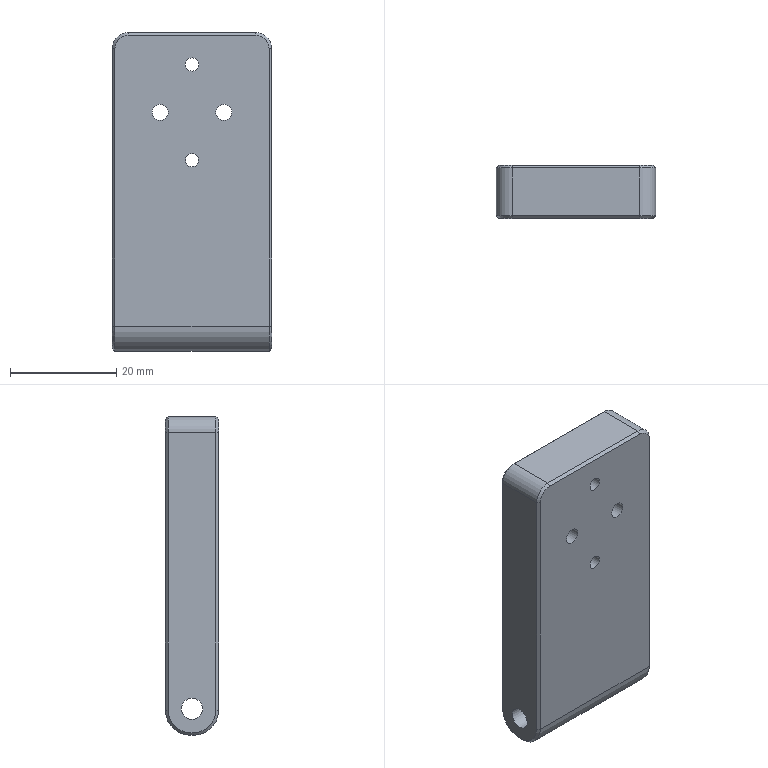Part | NX | 1 solid | 31 faces | box 30 x 10 x 60 mm | volume 17016 mm3 | plane 14 | cylinder 9 | cone 8 | commonest cylinder face diameters 2.5 x2 3 x2 6 x2 9.5 x2 4 x1
STEP:
#1=CARTESIAN_POINT('',(-12.,0.5,30.));
#2=VERTEX_POINT('',#1);
#3=CARTESIAN_POINT('',(-12.,0.,29.5));
#4=VERTEX_POINT('',#3);
#5=CARTESIAN_POINT('',(-12.,0.5,30.));
#6=DIRECTION('',(0.,-0.7071,-0.7071));
#7=VECTOR('',#6,1000.);
#8=LINE('',#5,#7);
#9=EDGE_CURVE('',#2,#4,#8,.T.);
#10=ORIENTED_EDGE('',*,*,#9,.T.);
#11=CARTESIAN_POINT('',(12.,0.,29.5));
#12=VERTEX_POINT('',#11);
#13=CARTESIAN_POINT('',(-12.,0.,29.5));
#14=DIRECTION('',(-1.,0.,0.));
#15=VECTOR('',#14,1000.);
#16=LINE('',#13,#15);
#17=EDGE_CURVE('',#12,#4,#16,.T.);
#18=ORIENTED_EDGE('',*,*,#17,.F.);
#19=CARTESIAN_POINT('',(12.,0.5,30.));
#20=VERTEX_POINT('',#19);
#21=CARTESIAN_POINT('',(12.,0.,29.5));
#22=DIRECTION('',(0.,0.7071,0.7071));
#23=VECTOR('',#22,1000.);
#24=LINE('',#21,#23);
#25=EDGE_CURVE('',#12,#20,#24,.T.);
#26=ORIENTED_EDGE('',*,*,#25,.T.);
#27=CARTESIAN_POINT('',(12.,0.5,30.));
#28=DIRECTION('',(1.,0.,0.));
#29=VECTOR('',#28,1000.);
#30=LINE('',#27,#29);
#31=EDGE_CURVE('',#2,#20,#30,.T.);
#32=ORIENTED_EDGE('',*,*,#31,.F.);
#33=EDGE_LOOP('',(#10,#18,#26,#32));
#34=FACE_BOUND('',#33,.T.);
#35=CARTESIAN_POINT('',(-15.,0.5,30.));
#36=DIRECTION('',(0.,-0.7071,0.7071));
#37=DIRECTION('',(-1.,0.,0.));
#38=AXIS2_PLACEMENT_3D('',#35,#36,#37);
#39=PLANE('',#38);
#40=ADVANCED_FACE('',(#34),#39,.T.);
#41=CARTESIAN_POINT('',(14.5,0.,27.));
#42=VERTEX_POINT('',#41);
#43=CARTESIAN_POINT('',(15.,0.5,27.));
#44=VERTEX_POINT('',#43);
#45=CARTESIAN_POINT('',(14.5,0.,27.));
#46=DIRECTION('',(0.7071,0.7071,0.));
#47=VECTOR('',#46,1000.);
#48=LINE('',#45,#47);
#49=EDGE_CURVE('',#42,#44,#48,.T.);
#50=ORIENTED_EDGE('',*,*,#49,.T.);
#51=CARTESIAN_POINT('',(12.,0.5,27.));
#52=DIRECTION('',(0.,1.,0.));
#53=DIRECTION('',(0.,0.,-1.));
#54=AXIS2_PLACEMENT_3D('',#51,#52,#53);
#55=CIRCLE('',#54,3.);
#56=EDGE_CURVE('',#20,#44,#55,.T.);
#57=ORIENTED_EDGE('',*,*,#56,.F.);
#58=ORIENTED_EDGE('',*,*,#25,.F.);
#59=CARTESIAN_POINT('',(12.,0.,27.));
#60=DIRECTION('',(0.,-1.,0.));
#61=DIRECTION('',(0.,0.,-1.));
#62=AXIS2_PLACEMENT_3D('',#59,#60,#61);
#63=CIRCLE('',#62,2.5);
#64=EDGE_CURVE('',#42,#12,#63,.T.);
#65=ORIENTED_EDGE('',*,*,#64,.F.);
#66=EDGE_LOOP('',(#50,#57,#58,#65));
#67=FACE_BOUND('',#66,.T.);
#68=CARTESIAN_POINT('',(12.,0.,27.));
#69=DIRECTION('',(0.,1.,0.));
#70=DIRECTION('',(0.,0.,1.));
#71=AXIS2_PLACEMENT_3D('',#68,#69,#70);
#72=CONICAL_SURFACE('',#71,2.5,0.7854);
#73=ADVANCED_FACE('',(#67),#72,.T.);
#74=CARTESIAN_POINT('',(-15.,0.5,27.));
#75=VERTEX_POINT('',#74);
#76=CARTESIAN_POINT('',(-14.5,0.,27.));
#77=VERTEX_POINT('',#76);
#78=CARTESIAN_POINT('',(-15.,0.5,27.));
#79=DIRECTION('',(0.7071,-0.7071,0.));
#80=VECTOR('',#79,1000.);
#81=LINE('',#78,#80);
#82=EDGE_CURVE('',#75,#77,#81,.T.);
#83=ORIENTED_EDGE('',*,*,#82,.T.);
#84=CARTESIAN_POINT('',(-12.,0.,27.));
#85=DIRECTION('',(0.,-1.,0.));
#86=DIRECTION('',(0.,0.,-1.));
#87=AXIS2_PLACEMENT_3D('',#84,#85,#86);
#88=CIRCLE('',#87,2.5);
#89=EDGE_CURVE('',#4,#77,#88,.T.);
#90=ORIENTED_EDGE('',*,*,#89,.F.);
#91=ORIENTED_EDGE('',*,*,#9,.F.);
#92=CARTESIAN_POINT('',(-12.,0.5,27.));
#93=DIRECTION('',(0.,1.,0.));
#94=DIRECTION('',(0.,0.,-1.));
#95=AXIS2_PLACEMENT_3D('',#92,#93,#94);
#96=CIRCLE('',#95,3.);
#97=EDGE_CURVE('',#75,#2,#96,.T.);
#98=ORIENTED_EDGE('',*,*,#97,.F.);
#99=EDGE_LOOP('',(#83,#90,#91,#98));
#100=FACE_BOUND('',#99,.T.);
#101=CARTESIAN_POINT('',(-12.,0.,27.));
#102=DIRECTION('',(0.,1.,0.));
#103=DIRECTION('',(0.,0.,1.));
#104=AXIS2_PLACEMENT_3D('',#101,#102,#103);
#105=CONICAL_SURFACE('',#104,2.5,0.7854);
#106=ADVANCED_FACE('',(#100),#105,.T.);
#107=CARTESIAN_POINT('',(14.5,0.,-25.25));
#108=VERTEX_POINT('',#107);
#109=CARTESIAN_POINT('',(15.,0.5,-25.25));
#110=VERTEX_POINT('',#109);
#111=CARTESIAN_POINT('',(14.5,0.,-25.25));
#112=DIRECTION('',(0.7071,0.7071,0.));
#113=VECTOR('',#112,1000.);
#114=LINE('',#111,#113);
#115=EDGE_CURVE('',#108,#110,#114,.T.);
#116=ORIENTED_EDGE('',*,*,#115,.T.);
#117=CARTESIAN_POINT('',(15.,0.5,-25.25));
#118=DIRECTION('',(0.,0.,-1.));
#119=VECTOR('',#118,1000.);
#120=LINE('',#117,#119);
#121=EDGE_CURVE('',#44,#110,#120,.T.);
#122=ORIENTED_EDGE('',*,*,#121,.F.);
#123=ORIENTED_EDGE('',*,*,#49,.F.);
#124=CARTESIAN_POINT('',(14.5,0.,27.));
#125=DIRECTION('',(0.,0.,1.));
#126=VECTOR('',#125,1000.);
#127=LINE('',#124,#126);
#128=EDGE_CURVE('',#108,#42,#127,.T.);
#129=ORIENTED_EDGE('',*,*,#128,.F.);
#130=EDGE_LOOP('',(#116,#122,#123,#129));
#131=FACE_BOUND('',#130,.T.);
#132=CARTESIAN_POINT('',(15.,0.5,30.));
#133=DIRECTION('',(0.7071,-0.7071,0.));
#134=DIRECTION('',(0.,0.,1.));
#135=AXIS2_PLACEMENT_3D('',#132,#133,#134);
#136=PLANE('',#135);
#137=ADVANCED_FACE('',(#131),#136,.T.);
#138=CARTESIAN_POINT('',(-15.,0.5,-25.25));
#139=VERTEX_POINT('',#138);
#140=CARTESIAN_POINT('',(-14.5,0.,-25.25));
#141=VERTEX_POINT('',#140);
#142=CARTESIAN_POINT('',(-15.,0.5,-25.25));
#143=DIRECTION('',(0.7071,-0.7071,0.));
#144=VECTOR('',#143,1000.);
#145=LINE('',#142,#144);
#146=EDGE_CURVE('',#139,#141,#145,.T.);
#147=ORIENTED_EDGE('',*,*,#146,.T.);
#148=CARTESIAN_POINT('',(-14.5,0.,-25.25));
#149=DIRECTION('',(0.,0.,-1.));
#150=VECTOR('',#149,1000.);
#151=LINE('',#148,#150);
#152=EDGE_CURVE('',#77,#141,#151,.T.);
#153=ORIENTED_EDGE('',*,*,#152,.F.);
#154=ORIENTED_EDGE('',*,*,#82,.F.);
#155=CARTESIAN_POINT('',(-15.,0.5,27.));
#156=DIRECTION('',(0.,0.,1.));
#157=VECTOR('',#156,1000.);
#158=LINE('',#155,#157);
#159=EDGE_CURVE('',#139,#75,#158,.T.);
#160=ORIENTED_EDGE('',*,*,#159,.F.);
#161=EDGE_LOOP('',(#147,#153,#154,#160));
#162=FACE_BOUND('',#161,.T.);
#163=CARTESIAN_POINT('',(-15.,0.5,30.));
#164=DIRECTION('',(-0.7071,-0.7071,0.));
#165=DIRECTION('',(0.,0.,-1.));
#166=AXIS2_PLACEMENT_3D('',#163,#164,#165);
#167=PLANE('',#166);
#168=ADVANCED_FACE('',(#162),#167,.T.);
#169=CARTESIAN_POINT('',(14.5,4.75,-30.));
#170=VERTEX_POINT('',#169);
#171=CARTESIAN_POINT('',(15.,4.75,-29.5));
#172=VERTEX_POINT('',#171);
#173=CARTESIAN_POINT('',(14.5,4.75,-30.));
#174=DIRECTION('',(0.7071,0.,0.7071));
#175=VECTOR('',#174,1000.);
#176=LINE('',#173,#175);
#177=EDGE_CURVE('',#170,#172,#176,.T.);
#178=ORIENTED_EDGE('',*,*,#177,.T.);
#179=CARTESIAN_POINT('',(15.,4.75,-25.25));
#180=DIRECTION('',(1.,0.,0.));
#181=DIRECTION('',(0.,0.,1.));
#182=AXIS2_PLACEMENT_3D('',#179,#180,#181);
#183=CIRCLE('',#182,4.25);
#184=EDGE_CURVE('',#110,#172,#183,.T.);
#185=ORIENTED_EDGE('',*,*,#184,.F.);
#186=ORIENTED_EDGE('',*,*,#115,.F.);
#187=CARTESIAN_POINT('',(14.5,4.75,-25.25));
#188=DIRECTION('',(-1.,0.,0.));
#189=DIRECTION('',(0.,0.,1.));
#190=AXIS2_PLACEMENT_3D('',#187,#188,#189);
#191=CIRCLE('',#190,4.75);
#192=EDGE_CURVE('',#170,#108,#191,.T.);
#193=ORIENTED_EDGE('',*,*,#192,.F.);
#194=EDGE_LOOP('',(#178,#185,#186,#193));
#195=FACE_BOUND('',#194,.T.);
#196=CARTESIAN_POINT('',(15.,4.75,-25.25));
#197=DIRECTION('',(-1.,0.,0.));
#198=DIRECTION('',(0.,0.,1.));
#199=AXIS2_PLACEMENT_3D('',#196,#197,#198);
#200=CONICAL_SURFACE('',#199,4.25,0.7854);
#201=ADVANCED_FACE('',(#195),#200,.T.);
#202=CARTESIAN_POINT('',(-15.,4.75,-29.5));
#203=VERTEX_POINT('',#202);
#204=CARTESIAN_POINT('',(-14.5,4.75,-30.));
#205=VERTEX_POINT('',#204);
#206=CARTESIAN_POINT('',(-15.,4.75,-29.5));
#207=DIRECTION('',(0.7071,0.,-0.7071));
#208=VECTOR('',#207,1000.);
#209=LINE('',#206,#208);
#210=EDGE_CURVE('',#203,#205,#209,.T.);
#211=ORIENTED_EDGE('',*,*,#210,.T.);
#212=CARTESIAN_POINT('',(-14.5,4.75,-25.25));
#213=DIRECTION('',(1.,0.,0.));
#214=DIRECTION('',(0.,0.,-1.));
#215=AXIS2_PLACEMENT_3D('',#212,#213,#214);
#216=CIRCLE('',#215,4.75);
#217=EDGE_CURVE('',#141,#205,#216,.T.);
#218=ORIENTED_EDGE('',*,*,#217,.F.);
#219=ORIENTED_EDGE('',*,*,#146,.F.);
#220=CARTESIAN_POINT('',(-15.,4.75,-25.25));
#221=DIRECTION('',(-1.,0.,0.));
#222=DIRECTION('',(0.,0.,-1.));
#223=AXIS2_PLACEMENT_3D('',#220,#221,#222);
#224=CIRCLE('',#223,4.25);
#225=EDGE_CURVE('',#203,#139,#224,.T.);
#226=ORIENTED_EDGE('',*,*,#225,.F.);
#227=EDGE_LOOP('',(#211,#218,#219,#226));
#228=FACE_BOUND('',#227,.T.);
#229=CARTESIAN_POINT('',(-15.,4.75,-25.25));
#230=DIRECTION('',(1.,0.,0.));
#231=DIRECTION('',(0.,0.,-1.));
#232=AXIS2_PLACEMENT_3D('',#229,#230,#231);
#233=CONICAL_SURFACE('',#232,4.25,0.7854);
#234=ADVANCED_FACE('',(#228),#233,.T.);
#235=CARTESIAN_POINT('',(14.5,5.25,-30.));
#236=VERTEX_POINT('',#235);
#237=CARTESIAN_POINT('',(15.,5.25,-29.5));
#238=VERTEX_POINT('',#237);
#239=CARTESIAN_POINT('',(14.5,5.25,-30.));
#240=DIRECTION('',(0.7071,0.,0.7071));
#241=VECTOR('',#240,1000.);
#242=LINE('',#239,#241);
#243=EDGE_CURVE('',#236,#238,#242,.T.);
#244=ORIENTED_EDGE('',*,*,#243,.T.);
#245=CARTESIAN_POINT('',(15.,10.,-29.5));
#246=DIRECTION('',(0.,1.,0.));
#247=VECTOR('',#246,1000.);
#248=LINE('',#245,#247);
#249=EDGE_CURVE('',#172,#238,#248,.T.);
#250=ORIENTED_EDGE('',*,*,#249,.F.);
#251=ORIENTED_EDGE('',*,*,#177,.F.);
#252=CARTESIAN_POINT('',(14.5,10.,-30.));
#253=DIRECTION('',(0.,-1.,0.));
#254=VECTOR('',#253,1000.);
#255=LINE('',#252,#254);
#256=EDGE_CURVE('',#236,#170,#255,.T.);
#257=ORIENTED_EDGE('',*,*,#256,.F.);
#258=EDGE_LOOP('',(#244,#250,#251,#257));
#259=FACE_BOUND('',#258,.T.);
#260=CARTESIAN_POINT('',(14.5,10.,-30.));
#261=DIRECTION('',(-0.7071,0.,0.7071));
#262=DIRECTION('',(0.,-1.,0.));
#263=AXIS2_PLACEMENT_3D('',#260,#261,#262);
#264=PLANE('',#263);
#265=ADVANCED_FACE('',(#259),#264,.F.);
#266=CARTESIAN_POINT('',(-15.,5.25,-29.5));
#267=VERTEX_POINT('',#266);
#268=CARTESIAN_POINT('',(-14.5,5.25,-30.));
#269=VERTEX_POINT('',#268);
#270=CARTESIAN_POINT('',(-15.,5.25,-29.5));
#271=DIRECTION('',(0.7071,0.,-0.7071));
#272=VECTOR('',#271,1000.);
#273=LINE('',#270,#272);
#274=EDGE_CURVE('',#267,#269,#273,.T.);
#275=ORIENTED_EDGE('',*,*,#274,.T.);
#276=CARTESIAN_POINT('',(-14.5,10.,-30.));
#277=DIRECTION('',(0.,1.,0.));
#278=VECTOR('',#277,1000.);
#279=LINE('',#276,#278);
#280=EDGE_CURVE('',#205,#269,#279,.T.);
#281=ORIENTED_EDGE('',*,*,#280,.F.);
#282=ORIENTED_EDGE('',*,*,#210,.F.);
#283=CARTESIAN_POINT('',(-15.,10.,-29.5));
#284=DIRECTION('',(0.,-1.,0.));
#285=VECTOR('',#284,1000.);
#286=LINE('',#283,#285);
#287=EDGE_CURVE('',#267,#203,#286,.T.);
#288=ORIENTED_EDGE('',*,*,#287,.F.);
#289=EDGE_LOOP('',(#275,#281,#282,#288));
#290=FACE_BOUND('',#289,.T.);
#291=CARTESIAN_POINT('',(-15.,10.,-29.5));
#292=DIRECTION('',(0.7071,0.,0.7071));
#293=DIRECTION('',(0.,-1.,0.));
#294=AXIS2_PLACEMENT_3D('',#291,#292,#293);
#295=PLANE('',#294);
#296=ADVANCED_FACE('',(#290),#295,.F.);
#297=CARTESIAN_POINT('',(14.5,10.,-25.25));
#298=VERTEX_POINT('',#297);
#299=CARTESIAN_POINT('',(15.,9.5,-25.25));
#300=VERTEX_POINT('',#299);
#301=CARTESIAN_POINT('',(14.5,10.,-25.25));
#302=DIRECTION('',(0.7071,-0.7071,0.));
#303=VECTOR('',#302,1000.);
#304=LINE('',#301,#303);
#305=EDGE_CURVE('',#298,#300,#304,.T.);
#306=ORIENTED_EDGE('',*,*,#305,.T.);
#307=CARTESIAN_POINT('',(15.,5.25,-25.25));
#308=DIRECTION('',(1.,0.,0.));
#309=DIRECTION('',(0.,0.,1.));
#310=AXIS2_PLACEMENT_3D('',#307,#308,#309);
#311=CIRCLE('',#310,4.25);
#312=EDGE_CURVE('',#238,#300,#311,.T.);
#313=ORIENTED_EDGE('',*,*,#312,.F.);
#314=ORIENTED_EDGE('',*,*,#243,.F.);
#315=CARTESIAN_POINT('',(14.5,5.25,-25.25));
#316=DIRECTION('',(-1.,0.,0.));
#317=DIRECTION('',(0.,0.,1.));
#318=AXIS2_PLACEMENT_3D('',#315,#316,#317);
#319=CIRCLE('',#318,4.75);
#320=EDGE_CURVE('',#298,#236,#319,.T.);
#321=ORIENTED_EDGE('',*,*,#320,.F.);
#322=EDGE_LOOP('',(#306,#313,#314,#321));
#323=FACE_BOUND('',#322,.T.);
#324=CARTESIAN_POINT('',(15.,5.25,-25.25));
#325=DIRECTION('',(-1.,0.,0.));
#326=DIRECTION('',(0.,0.,1.));
#327=AXIS2_PLACEMENT_3D('',#324,#325,#326);
#328=CONICAL_SURFACE('',#327,4.25,0.7854);
#329=ADVANCED_FACE('',(#323),#328,.T.);
#330=CARTESIAN_POINT('',(-15.,9.5,-25.25));
#331=VERTEX_POINT('',#330);
#332=CARTESIAN_POINT('',(-14.5,10.,-25.25));
#333=VERTEX_POINT('',#332);
#334=CARTESIAN_POINT('',(-15.,9.5,-25.25));
#335=DIRECTION('',(0.7071,0.7071,0.));
#336=VECTOR('',#335,1000.);
#337=LINE('',#334,#336);
#338=EDGE_CURVE('',#331,#333,#337,.T.);
#339=ORIENTED_EDGE('',*,*,#338,.T.);
#340=CARTESIAN_POINT('',(-14.5,5.25,-25.25));
#341=DIRECTION('',(1.,0.,0.));
#342=DIRECTION('',(0.,0.,-1.));
#343=AXIS2_PLACEMENT_3D('',#340,#341,#342);
#344=CIRCLE('',#343,4.75);
#345=EDGE_CURVE('',#269,#333,#344,.T.);
#346=ORIENTED_EDGE('',*,*,#345,.F.);
#347=ORIENTED_EDGE('',*,*,#274,.F.);
#348=CARTESIAN_POINT('',(-15.,5.25,-25.25));
#349=DIRECTION('',(-1.,0.,0.));
#350=DIRECTION('',(0.,0.,-1.));
#351=AXIS2_PLACEMENT_3D('',#348,#349,#350);
#352=CIRCLE('',#351,4.25);
#353=EDGE_CURVE('',#331,#267,#352,.T.);
#354=ORIENTED_EDGE('',*,*,#353,.F.);
#355=EDGE_LOOP('',(#339,#346,#347,#354));
#356=FACE_BOUND('',#355,.T.);
#357=CARTESIAN_POINT('',(-15.,5.25,-25.25));
#358=DIRECTION('',(1.,0.,0.));
#359=DIRECTION('',(0.,0.,-1.));
#360=AXIS2_PLACEMENT_3D('',#357,#358,#359);
#361=CONICAL_SURFACE('',#360,4.25,0.7854);
#362=ADVANCED_FACE('',(#356),#361,.T.);
#363=CARTESIAN_POINT('',(14.5,10.,27.));
#364=VERTEX_POINT('',#363);
#365=CARTESIAN_POINT('',(15.,9.5,27.));
#366=VERTEX_POINT('',#365);
#367=CARTESIAN_POINT('',(14.5,10.,27.));
#368=DIRECTION('',(0.7071,-0.7071,0.));
#369=VECTOR('',#368,1000.);
#370=LINE('',#367,#369);
#371=EDGE_CURVE('',#364,#366,#370,.T.);
#372=ORIENTED_EDGE('',*,*,#371,.T.);
#373=CARTESIAN_POINT('',(15.,9.5,30.));
#374=DIRECTION('',(0.,0.,1.));
#375=VECTOR('',#374,1000.);
#376=LINE('',#373,#375);
#377=EDGE_CURVE('',#300,#366,#376,.T.);
#378=ORIENTED_EDGE('',*,*,#377,.F.);
#379=ORIENTED_EDGE('',*,*,#305,.F.);
#380=CARTESIAN_POINT('',(14.5,10.,0.));
#381=DIRECTION('',(0.,0.,-1.));
#382=VECTOR('',#381,1000.);
#383=LINE('',#380,#382);
#384=EDGE_CURVE('',#364,#298,#383,.T.);
#385=ORIENTED_EDGE('',*,*,#384,.F.);
#386=EDGE_LOOP('',(#372,#378,#379,#385));
#387=FACE_BOUND('',#386,.T.);
#388=CARTESIAN_POINT('',(14.5,10.,0.));
#389=DIRECTION('',(-0.7071,-0.7071,0.));
#390=DIRECTION('',(0.,0.,-1.));
#391=AXIS2_PLACEMENT_3D('',#388,#389,#390);
#392=PLANE('',#391);
#393=ADVANCED_FACE('',(#387),#392,.F.);
#394=CARTESIAN_POINT('',(-15.,9.5,27.));
#395=VERTEX_POINT('',#394);
#396=CARTESIAN_POINT('',(-14.5,10.,27.));
#397=VERTEX_POINT('',#396);
#398=CARTESIAN_POINT('',(-15.,9.5,27.));
#399=DIRECTION('',(0.7071,0.7071,0.));
#400=VECTOR('',#399,1000.);
#401=LINE('',#398,#400);
#402=EDGE_CURVE('',#395,#397,#401,.T.);
#403=ORIENTED_EDGE('',*,*,#402,.T.);
#404=CARTESIAN_POINT('',(-14.5,10.,0.));
#405=DIRECTION('',(0.,0.,1.));
#406=VECTOR('',#405,1000.);
#407=LINE('',#404,#406);
#408=EDGE_CURVE('',#333,#397,#407,.T.);
#409=ORIENTED_EDGE('',*,*,#408,.F.);
#410=ORIENTED_EDGE('',*,*,#338,.F.);
#411=CARTESIAN_POINT('',(-15.,9.5,30.));
#412=DIRECTION('',(0.,0.,-1.));
#413=VECTOR('',#412,1000.);
#414=LINE('',#411,#413);
#415=EDGE_CURVE('',#395,#331,#414,.T.);
#416=ORIENTED_EDGE('',*,*,#415,.F.);
#417=EDGE_LOOP('',(#403,#409,#410,#416));
#418=FACE_BOUND('',#417,.T.);
#419=CARTESIAN_POINT('',(-14.5,10.,0.));
#420=DIRECTION('',(0.7071,-0.7071,0.));
#421=DIRECTION('',(0.,0.,1.));
#422=AXIS2_PLACEMENT_3D('',#419,#420,#421);
#423=PLANE('',#422);
#424=ADVANCED_FACE('',(#418),#423,.F.);
#425=CARTESIAN_POINT('',(12.,10.,29.5));
#426=VERTEX_POINT('',#425);
#427=CARTESIAN_POINT('',(12.,9.5,30.));
#428=VERTEX_POINT('',#427);
#429=CARTESIAN_POINT('',(12.,10.,29.5));
#430=DIRECTION('',(0.,-0.7071,0.7071));
#431=VECTOR('',#430,1000.);
#432=LINE('',#429,#431);
#433=EDGE_CURVE('',#426,#428,#432,.T.);
#434=ORIENTED_EDGE('',*,*,#433,.T.);
#435=CARTESIAN_POINT('',(12.,9.5,27.));
#436=DIRECTION('',(0.,-1.,0.));
#437=DIRECTION('',(0.,0.,-1.));
#438=AXIS2_PLACEMENT_3D('',#435,#436,#437);
#439=CIRCLE('',#438,3.);
#440=EDGE_CURVE('',#366,#428,#439,.T.);
#441=ORIENTED_EDGE('',*,*,#440,.F.);
#442=ORIENTED_EDGE('',*,*,#371,.F.);
#443=CARTESIAN_POINT('',(12.,10.,27.));
#444=DIRECTION('',(0.,1.,0.));
#445=DIRECTION('',(0.,0.,-1.));
#446=AXIS2_PLACEMENT_3D('',#443,#444,#445);
#447=CIRCLE('',#446,2.5);
#448=EDGE_CURVE('',#426,#364,#447,.T.);
#449=ORIENTED_EDGE('',*,*,#448,.F.);
#450=EDGE_LOOP('',(#434,#441,#442,#449));
#451=FACE_BOUND('',#450,.T.);
#452=CARTESIAN_POINT('',(12.,10.,27.));
#453=DIRECTION('',(0.,-1.,0.));
#454=DIRECTION('',(0.,0.,-1.));
#455=AXIS2_PLACEMENT_3D('',#452,#453,#454);
#456=CONICAL_SURFACE('',#455,2.5,0.7854);
#457=ADVANCED_FACE('',(#451),#456,.T.);
#458=CARTESIAN_POINT('',(-12.,9.5,30.));
#459=VERTEX_POINT('',#458);
#460=CARTESIAN_POINT('',(-12.,10.,29.5));
#461=VERTEX_POINT('',#460);
#462=CARTESIAN_POINT('',(-12.,9.5,30.));
#463=DIRECTION('',(0.,0.7071,-0.7071));
#464=VECTOR('',#463,1000.);
#465=LINE('',#462,#464);
#466=EDGE_CURVE('',#459,#461,#465,.T.);
#467=ORIENTED_EDGE('',*,*,#466,.T.);
#468=CARTESIAN_POINT('',(-12.,10.,27.));
#469=DIRECTION('',(0.,1.,0.));
#470=DIRECTION('',(0.,0.,-1.));
#471=AXIS2_PLACEMENT_3D('',#468,#469,#470);
#472=CIRCLE('',#471,2.5);
#473=EDGE_CURVE('',#397,#461,#472,.T.);
#474=ORIENTED_EDGE('',*,*,#473,.F.);
#475=ORIENTED_EDGE('',*,*,#402,.F.);
#476=CARTESIAN_POINT('',(-12.,9.5,27.));
#477=DIRECTION('',(0.,-1.,0.));
#478=DIRECTION('',(0.,0.,-1.));
#479=AXIS2_PLACEMENT_3D('',#476,#477,#478);
#480=CIRCLE('',#479,3.);
#481=EDGE_CURVE('',#459,#395,#480,.T.);
#482=ORIENTED_EDGE('',*,*,#481,.F.);
#483=EDGE_LOOP('',(#467,#474,#475,#482));
#484=FACE_BOUND('',#483,.T.);
#485=CARTESIAN_POINT('',(-12.,10.,27.));
#486=DIRECTION('',(0.,-1.,0.));
#487=DIRECTION('',(0.,0.,-1.));
#488=AXIS2_PLACEMENT_3D('',#485,#486,#487);
#489=CONICAL_SURFACE('',#488,2.5,0.7854);
#490=ADVANCED_FACE('',(#484),#489,.T.);
#491=ORIENTED_EDGE('',*,*,#433,.F.);
#492=CARTESIAN_POINT('',(0.,10.,29.5));
#493=DIRECTION('',(1.,0.,0.));
#494=VECTOR('',#493,1000.);
#495=LINE('',#492,#494);
#496=EDGE_CURVE('',#461,#426,#495,.T.);
#497=ORIENTED_EDGE('',*,*,#496,.F.);
#498=ORIENTED_EDGE('',*,*,#466,.F.);
#499=CARTESIAN_POINT('',(-15.,9.5,30.));
#500=DIRECTION('',(-1.,0.,0.));
#501=VECTOR('',#500,1000.);
#502=LINE('',#499,#501);
#503=EDGE_CURVE('',#428,#459,#502,.T.);
#504=ORIENTED_EDGE('',*,*,#503,.F.);
#505=EDGE_LOOP('',(#491,#497,#498,#504));
#506=FACE_BOUND('',#505,.T.);
#507=CARTESIAN_POINT('',(0.,10.,29.5));
#508=DIRECTION('',(0.,-0.7071,-0.7071));
#509=DIRECTION('',(1.,0.,0.));
#510=AXIS2_PLACEMENT_3D('',#507,#508,#509);
#511=PLANE('',#510);
#512=ADVANCED_FACE('',(#506),#511,.F.);
#513=CARTESIAN_POINT('',(-15.,10.,27.));
#514=DIRECTION('',(0.,1.,0.));
#515=VECTOR('',#514,1000.);
#516=LINE('',#513,#515);
#517=EDGE_CURVE('',#75,#395,#516,.T.);
#518=ORIENTED_EDGE('',*,*,#517,.F.);
#519=ORIENTED_EDGE('',*,*,#97,.T.);
#520=CARTESIAN_POINT('',(-12.,10.,30.));
#521=DIRECTION('',(0.,-1.,0.));
#522=VECTOR('',#521,1000.);
#523=LINE('',#520,#522);
#524=EDGE_CURVE('',#459,#2,#523,.T.);
#525=ORIENTED_EDGE('',*,*,#524,.F.);
#526=ORIENTED_EDGE('',*,*,#481,.T.);
#527=EDGE_LOOP('',(#518,#519,#525,#526));
#528=FACE_BOUND('',#527,.T.);
#529=CARTESIAN_POINT('',(-12.,10.,27.));
#530=DIRECTION('',(0.,-1.,0.));
#531=DIRECTION('',(0.,0.,-1.));
#532=AXIS2_PLACEMENT_3D('',#529,#530,#531);
#533=CYLINDRICAL_SURFACE('',#532,3.);
#534=ADVANCED_FACE('',(#528),#533,.T.);
#535=CARTESIAN_POINT('',(12.,10.,30.));
#536=DIRECTION('',(0.,1.,0.));
#537=VECTOR('',#536,1000.);
#538=LINE('',#535,#537);
#539=EDGE_CURVE('',#20,#428,#538,.T.);
#540=ORIENTED_EDGE('',*,*,#539,.F.);
#541=ORIENTED_EDGE('',*,*,#56,.T.);
#542=CARTESIAN_POINT('',(15.,10.,27.));
#543=DIRECTION('',(0.,-1.,0.));
#544=VECTOR('',#543,1000.);
#545=LINE('',#542,#544);
#546=EDGE_CURVE('',#366,#44,#545,.T.);
#547=ORIENTED_EDGE('',*,*,#546,.F.);
#548=ORIENTED_EDGE('',*,*,#440,.T.);
#549=EDGE_LOOP('',(#540,#541,#547,#548));
#550=FACE_BOUND('',#549,.T.);
#551=CARTESIAN_POINT('',(12.,10.,27.));
#552=DIRECTION('',(0.,-1.,0.));
#553=DIRECTION('',(0.,0.,-1.));
#554=AXIS2_PLACEMENT_3D('',#551,#552,#553);
#555=CYLINDRICAL_SURFACE('',#554,3.);
#556=ADVANCED_FACE('',(#550),#555,.T.);
#557=CARTESIAN_POINT('',(-15.,5.25,-30.));
#558=DIRECTION('',(1.,0.,0.));
#559=VECTOR('',#558,1000.);
#560=LINE('',#557,#559);
#561=EDGE_CURVE('',#269,#236,#560,.T.);
#562=ORIENTED_EDGE('',*,*,#561,.F.);
#563=ORIENTED_EDGE('',*,*,#345,.T.);
#564=CARTESIAN_POINT('',(0.,10.,-25.25));
#565=DIRECTION('',(-1.,0.,0.));
#566=VECTOR('',#565,1000.);
#567=LINE('',#564,#566);
#568=EDGE_CURVE('',#298,#333,#567,.T.);
#569=ORIENTED_EDGE('',*,*,#568,.F.);
#570=ORIENTED_EDGE('',*,*,#320,.T.);
#571=EDGE_LOOP('',(#562,#563,#569,#570));
#572=FACE_BOUND('',#571,.T.);
#573=CARTESIAN_POINT('',(0.,5.25,-25.25));
#574=DIRECTION('',(-1.,0.,0.));
#575=DIRECTION('',(0.,0.,1.));
#576=AXIS2_PLACEMENT_3D('',#573,#574,#575);
#577=CYLINDRICAL_SURFACE('',#576,4.75);
#578=ADVANCED_FACE('',(#572),#577,.T.);
#579=CARTESIAN_POINT('',(15.,0.,-25.25));
#580=DIRECTION('',(1.,0.,0.));
#581=VECTOR('',#580,1000.);
#582=LINE('',#579,#581);
#583=EDGE_CURVE('',#141,#108,#582,.T.);
#584=ORIENTED_EDGE('',*,*,#583,.F.);
#585=ORIENTED_EDGE('',*,*,#217,.T.);
#586=CARTESIAN_POINT('',(-15.,4.75,-30.));
#587=DIRECTION('',(-1.,0.,0.));
#588=VECTOR('',#587,1000.);
#589=LINE('',#586,#588);
#590=EDGE_CURVE('',#170,#205,#589,.T.);
#591=ORIENTED_EDGE('',*,*,#590,.F.);
#592=ORIENTED_EDGE('',*,*,#192,.T.);
#593=EDGE_LOOP('',(#584,#585,#591,#592));
#594=FACE_BOUND('',#593,.T.);
#595=CARTESIAN_POINT('',(-15.,4.75,-25.25));
#596=DIRECTION('',(1.,0.,0.));
#597=DIRECTION('',(0.,0.,-1.));
#598=AXIS2_PLACEMENT_3D('',#595,#596,#597);
#599=CYLINDRICAL_SURFACE('',#598,4.75);
#600=ADVANCED_FACE('',(#594),#599,.T.);
#601=ORIENTED_EDGE('',*,*,#89,.T.);
#602=ORIENTED_EDGE('',*,*,#152,.T.);
#603=ORIENTED_EDGE('',*,*,#583,.T.);
#604=ORIENTED_EDGE('',*,*,#128,.T.);
#605=ORIENTED_EDGE('',*,*,#64,.T.);
#606=ORIENTED_EDGE('',*,*,#17,.T.);
#607=EDGE_LOOP('',(#601,#602,#603,#604,#605,#606));
#608=FACE_BOUND('',#607,.T.);
#609=CARTESIAN_POINT('',(0.,0.,22.75));
#610=VERTEX_POINT('',#609);
#611=CARTESIAN_POINT('',(0.,0.,24.));
#612=DIRECTION('',(0.,-1.,0.));
#613=DIRECTION('',(0.,0.,-1.));
#614=AXIS2_PLACEMENT_3D('',#611,#612,#613);
#615=CIRCLE('',#614,1.25);
#616=EDGE_CURVE('',#610,#610,#615,.T.);
#617=ORIENTED_EDGE('',*,*,#616,.F.);
#618=EDGE_LOOP('',(#617));
#619=FACE_BOUND('',#618,.T.);
#620=CARTESIAN_POINT('',(0.,0.,4.75));
#621=VERTEX_POINT('',#620);
#622=CARTESIAN_POINT('',(0.,0.,6.));
#623=DIRECTION('',(0.,-1.,0.));
#624=DIRECTION('',(0.,0.,-1.));
#625=AXIS2_PLACEMENT_3D('',#622,#623,#624);
#626=CIRCLE('',#625,1.25);
#627=EDGE_CURVE('',#621,#621,#626,.T.);
#628=ORIENTED_EDGE('',*,*,#627,.F.);
#629=EDGE_LOOP('',(#628));
#630=FACE_BOUND('',#629,.T.);
#631=CARTESIAN_POINT('',(6.,0.,13.5));
#632=VERTEX_POINT('',#631);
#633=CARTESIAN_POINT('',(6.,0.,15.));
#634=DIRECTION('',(0.,-1.,0.));
#635=DIRECTION('',(0.,0.,-1.));
#636=AXIS2_PLACEMENT_3D('',#633,#634,#635);
#637=CIRCLE('',#636,1.5);
#638=EDGE_CURVE('',#632,#632,#637,.T.);
#639=ORIENTED_EDGE('',*,*,#638,.F.);
#640=EDGE_LOOP('',(#639));
#641=FACE_BOUND('',#640,.T.);
#642=CARTESIAN_POINT('',(-6.,0.,13.5));
#643=VERTEX_POINT('',#642);
#644=CARTESIAN_POINT('',(-6.,0.,15.));
#645=DIRECTION('',(0.,-1.,0.));
#646=DIRECTION('',(0.,0.,-1.));
#647=AXIS2_PLACEMENT_3D('',#644,#645,#646);
#648=CIRCLE('',#647,1.5);
#649=EDGE_CURVE('',#643,#643,#648,.T.);
#650=ORIENTED_EDGE('',*,*,#649,.F.);
#651=EDGE_LOOP('',(#650));
#652=FACE_BOUND('',#651,.T.);
#653=CARTESIAN_POINT('',(0.,0.,0.));
#654=DIRECTION('',(0.,-1.,0.));
#655=DIRECTION('',(0.,0.,-1.));
#656=AXIS2_PLACEMENT_3D('',#653,#654,#655);
#657=PLANE('',#656);
#658=ADVANCED_FACE('',(#608,#619,#630,#641,#652),#657,.T.);
#659=ORIENTED_EDGE('',*,*,#568,.T.);
#660=ORIENTED_EDGE('',*,*,#408,.T.);
#661=ORIENTED_EDGE('',*,*,#473,.T.);
#662=ORIENTED_EDGE('',*,*,#496,.T.);
#663=ORIENTED_EDGE('',*,*,#448,.T.);
#664=ORIENTED_EDGE('',*,*,#384,.T.);
#665=EDGE_LOOP('',(#659,#660,#661,#662,#663,#664));
#666=FACE_BOUND('',#665,.T.);
#667=CARTESIAN_POINT('',(0.,10.,25.25));
#668=VERTEX_POINT('',#667);
#669=CARTESIAN_POINT('',(0.,10.,24.));
#670=DIRECTION('',(0.,1.,0.));
#671=DIRECTION('',(0.,0.,1.));
#672=AXIS2_PLACEMENT_3D('',#669,#670,#671);
#673=CIRCLE('',#672,1.25);
#674=EDGE_CURVE('',#668,#668,#673,.T.);
#675=ORIENTED_EDGE('',*,*,#674,.F.);
#676=EDGE_LOOP('',(#675));
#677=FACE_BOUND('',#676,.T.);
#678=CARTESIAN_POINT('',(0.,10.,7.25));
#679=VERTEX_POINT('',#678);
#680=CARTESIAN_POINT('',(0.,10.,6.));
#681=DIRECTION('',(0.,1.,0.));
#682=DIRECTION('',(0.,0.,1.));
#683=AXIS2_PLACEMENT_3D('',#680,#681,#682);
#684=CIRCLE('',#683,1.25);
#685=EDGE_CURVE('',#679,#679,#684,.T.);
#686=ORIENTED_EDGE('',*,*,#685,.F.);
#687=EDGE_LOOP('',(#686));
#688=FACE_BOUND('',#687,.T.);
#689=CARTESIAN_POINT('',(6.,10.,16.5));
#690=VERTEX_POINT('',#689);
#691=CARTESIAN_POINT('',(6.,10.,15.));
#692=DIRECTION('',(0.,1.,0.));
#693=DIRECTION('',(0.,0.,1.));
#694=AXIS2_PLACEMENT_3D('',#691,#692,#693);
#695=CIRCLE('',#694,1.5);
#696=EDGE_CURVE('',#690,#690,#695,.T.);
#697=ORIENTED_EDGE('',*,*,#696,.F.);
#698=EDGE_LOOP('',(#697));
#699=FACE_BOUND('',#698,.T.);
#700=CARTESIAN_POINT('',(-6.,10.,16.5));
#701=VERTEX_POINT('',#700);
#702=CARTESIAN_POINT('',(-6.,10.,15.));
#703=DIRECTION('',(0.,1.,0.));
#704=DIRECTION('',(0.,0.,1.));
#705=AXIS2_PLACEMENT_3D('',#702,#703,#704);
#706=CIRCLE('',#705,1.5);
#707=EDGE_CURVE('',#701,#701,#706,.T.);
#708=ORIENTED_EDGE('',*,*,#707,.F.);
#709=EDGE_LOOP('',(#708));
#710=FACE_BOUND('',#709,.T.);
#711=CARTESIAN_POINT('',(0.,10.,0.));
#712=DIRECTION('',(0.,-1.,0.));
#713=DIRECTION('',(0.,0.,-1.));
#714=AXIS2_PLACEMENT_3D('',#711,#712,#713);
#715=PLANE('',#714);
#716=ADVANCED_FACE('',(#666,#677,#688,#699,#710),#715,.F.);
#717=ORIENTED_EDGE('',*,*,#524,.T.);
#718=ORIENTED_EDGE('',*,*,#31,.T.);
#719=ORIENTED_EDGE('',*,*,#539,.T.);
#720=ORIENTED_EDGE('',*,*,#503,.T.);
#721=EDGE_LOOP('',(#717,#718,#719,#720));
#722=FACE_BOUND('',#721,.T.);
#723=CARTESIAN_POINT('',(-15.,10.,30.));
#724=DIRECTION('',(0.,0.,-1.));
#725=DIRECTION('',(-1.,0.,0.));
#726=AXIS2_PLACEMENT_3D('',#723,#724,#725);
#727=PLANE('',#726);
#728=ADVANCED_FACE('',(#722),#727,.F.);
#729=ORIENTED_EDGE('',*,*,#225,.T.);
#730=ORIENTED_EDGE('',*,*,#159,.T.);
#731=ORIENTED_EDGE('',*,*,#517,.T.);
#732=ORIENTED_EDGE('',*,*,#415,.T.);
#733=ORIENTED_EDGE('',*,*,#353,.T.);
#734=ORIENTED_EDGE('',*,*,#287,.T.);
#735=EDGE_LOOP('',(#729,#730,#731,#732,#733,#734));
#736=FACE_BOUND('',#735,.T.);
#737=CARTESIAN_POINT('',(-15.,5.,-23.));
#738=VERTEX_POINT('',#737);
#739=CARTESIAN_POINT('',(-15.,5.,-25.));
#740=DIRECTION('',(-1.,0.,0.));
#741=DIRECTION('',(0.,0.,1.));
#742=AXIS2_PLACEMENT_3D('',#739,#740,#741);
#743=CIRCLE('',#742,2.);
#744=EDGE_CURVE('',#738,#738,#743,.T.);
#745=ORIENTED_EDGE('',*,*,#744,.F.);
#746=EDGE_LOOP('',(#745));
#747=FACE_BOUND('',#746,.T.);
#748=CARTESIAN_POINT('',(-15.,10.,30.));
#749=DIRECTION('',(1.,0.,0.));
#750=DIRECTION('',(0.,0.,-1.));
#751=AXIS2_PLACEMENT_3D('',#748,#749,#750);
#752=PLANE('',#751);
#753=ADVANCED_FACE('',(#736,#747),#752,.F.);
#754=ORIENTED_EDGE('',*,*,#590,.T.);
#755=ORIENTED_EDGE('',*,*,#280,.T.);
#756=ORIENTED_EDGE('',*,*,#561,.T.);
#757=ORIENTED_EDGE('',*,*,#256,.T.);
#758=EDGE_LOOP('',(#754,#755,#756,#757));
#759=FACE_BOUND('',#758,.T.);
#760=CARTESIAN_POINT('',(-15.,10.,-30.));
#761=DIRECTION('',(0.,0.,1.));
#762=DIRECTION('',(1.,0.,0.));
#763=AXIS2_PLACEMENT_3D('',#760,#761,#762);
#764=PLANE('',#763);
#765=ADVANCED_FACE('',(#759),#764,.F.);
#766=ORIENTED_EDGE('',*,*,#546,.T.);
#767=ORIENTED_EDGE('',*,*,#121,.T.);
#768=ORIENTED_EDGE('',*,*,#184,.T.);
#769=ORIENTED_EDGE('',*,*,#249,.T.);
#770=ORIENTED_EDGE('',*,*,#312,.T.);
#771=ORIENTED_EDGE('',*,*,#377,.T.);
#772=EDGE_LOOP('',(#766,#767,#768,#769,#770,#771));
#773=FACE_BOUND('',#772,.T.);
#774=CARTESIAN_POINT('',(15.,5.,-23.));
#775=VERTEX_POINT('',#774);
#776=CARTESIAN_POINT('',(15.,5.,-25.));
#777=DIRECTION('',(-1.,0.,0.));
#778=DIRECTION('',(0.,0.,1.));
#779=AXIS2_PLACEMENT_3D('',#776,#777,#778);
#780=CIRCLE('',#779,2.);
#781=EDGE_CURVE('',#775,#775,#780,.T.);
#782=ORIENTED_EDGE('',*,*,#781,.T.);
#783=EDGE_LOOP('',(#782));
#784=FACE_BOUND('',#783,.T.);
#785=CARTESIAN_POINT('',(15.,10.,30.));
#786=DIRECTION('',(-1.,0.,0.));
#787=DIRECTION('',(0.,0.,1.));
#788=AXIS2_PLACEMENT_3D('',#785,#786,#787);
#789=PLANE('',#788);
#790=ADVANCED_FACE('',(#773,#784),#789,.F.);
#791=ORIENTED_EDGE('',*,*,#781,.F.);
#792=EDGE_LOOP('',(#791));
#793=FACE_BOUND('',#792,.T.);
#794=ORIENTED_EDGE('',*,*,#744,.T.);
#795=EDGE_LOOP('',(#794));
#796=FACE_BOUND('',#795,.T.);
#797=CARTESIAN_POINT('',(-15.,5.,-25.));
#798=DIRECTION('',(-1.,0.,0.));
#799=DIRECTION('',(0.,0.,1.));
#800=AXIS2_PLACEMENT_3D('',#797,#798,#799);
#801=CYLINDRICAL_SURFACE('',#800,2.);
#802=ADVANCED_FACE('',(#793,#796),#801,.F.);
#803=ORIENTED_EDGE('',*,*,#616,.T.);
#804=EDGE_LOOP('',(#803));
#805=FACE_BOUND('',#804,.T.);
#806=ORIENTED_EDGE('',*,*,#674,.T.);
#807=EDGE_LOOP('',(#806));
#808=FACE_BOUND('',#807,.T.);
#809=CARTESIAN_POINT('',(0.,10.,24.));
#810=DIRECTION('',(0.,1.,0.));
#811=DIRECTION('',(0.,0.,1.));
#812=AXIS2_PLACEMENT_3D('',#809,#810,#811);
#813=CYLINDRICAL_SURFACE('',#812,1.25);
#814=ADVANCED_FACE('',(#805,#808),#813,.F.);
#815=ORIENTED_EDGE('',*,*,#627,.T.);
#816=EDGE_LOOP('',(#815));
#817=FACE_BOUND('',#816,.T.);
#818=ORIENTED_EDGE('',*,*,#685,.T.);
#819=EDGE_LOOP('',(#818));
#820=FACE_BOUND('',#819,.T.);
#821=CARTESIAN_POINT('',(0.,10.,6.));
#822=DIRECTION('',(0.,1.,0.));
#823=DIRECTION('',(0.,0.,1.));
#824=AXIS2_PLACEMENT_3D('',#821,#822,#823);
#825=CYLINDRICAL_SURFACE('',#824,1.25);
#826=ADVANCED_FACE('',(#817,#820),#825,.F.);
#827=ORIENTED_EDGE('',*,*,#638,.T.);
#828=EDGE_LOOP('',(#827));
#829=FACE_BOUND('',#828,.T.);
#830=ORIENTED_EDGE('',*,*,#696,.T.);
#831=EDGE_LOOP('',(#830));
#832=FACE_BOUND('',#831,.T.);
#833=CARTESIAN_POINT('',(6.,10.,15.));
#834=DIRECTION('',(0.,1.,0.));
#835=DIRECTION('',(0.,0.,1.));
#836=AXIS2_PLACEMENT_3D('',#833,#834,#835);
#837=CYLINDRICAL_SURFACE('',#836,1.5);
#838=ADVANCED_FACE('',(#829,#832),#837,.F.);
#839=ORIENTED_EDGE('',*,*,#649,.T.);
#840=EDGE_LOOP('',(#839));
#841=FACE_BOUND('',#840,.T.);
#842=ORIENTED_EDGE('',*,*,#707,.T.);
#843=EDGE_LOOP('',(#842));
#844=FACE_BOUND('',#843,.T.);
#845=CARTESIAN_POINT('',(-6.,10.,15.));
#846=DIRECTION('',(0.,1.,0.));
#847=DIRECTION('',(0.,0.,1.));
#848=AXIS2_PLACEMENT_3D('',#845,#846,#847);
#849=CYLINDRICAL_SURFACE('',#848,1.5);
#850=ADVANCED_FACE('',(#841,#844),#849,.F.);
#851=CLOSED_SHELL('',(#40,#73,#106,#137,#168,#201,#234,#265,#296,#329,#362,#393,#424,#457,#490,#512,#534,#556,#578,#600,#658,#716,#728,#753,#765,#790,#802,#814,#826,#838,#850));
#852=MANIFOLD_SOLID_BREP('',#851);
#853=(LENGTH_UNIT()NAMED_UNIT(*)SI_UNIT(.MILLI.,.METRE.));
#854=UNCERTAINTY_MEASURE_WITH_UNIT(LENGTH_MEASURE(0.00001),#853,'','');
#855=(NAMED_UNIT(*)PLANE_ANGLE_UNIT()SI_UNIT($,.RADIAN.));
#856=(NAMED_UNIT(*)SI_UNIT($,.STERADIAN.)SOLID_ANGLE_UNIT());
#857=(GEOMETRIC_REPRESENTATION_CONTEXT(3)GLOBAL_UNCERTAINTY_ASSIGNED_CONTEXT((#854))GLOBAL_UNIT_ASSIGNED_CONTEXT((#853,#855,#856))REPRESENTATION_CONTEXT('',''));
#858=ADVANCED_BREP_SHAPE_REPRESENTATION('',(#852),#857);